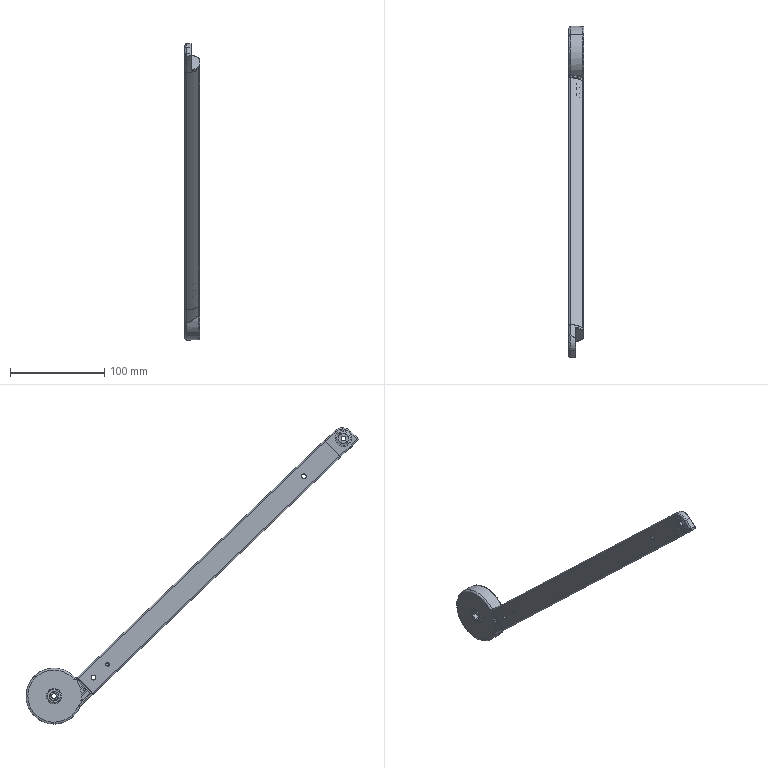Part | SolidWorks | 3 solids | 573 faces | box 16.903 x 352.818 x 314.841 mm | volume 72697 mm3 | plane 312 | cylinder 178 | spline 77 | cone 6 | commonest cylinder face diameters 3.137 x18 53.372 x17 0.98 x15 44.411 x9 1.961 x8 5.2 x8